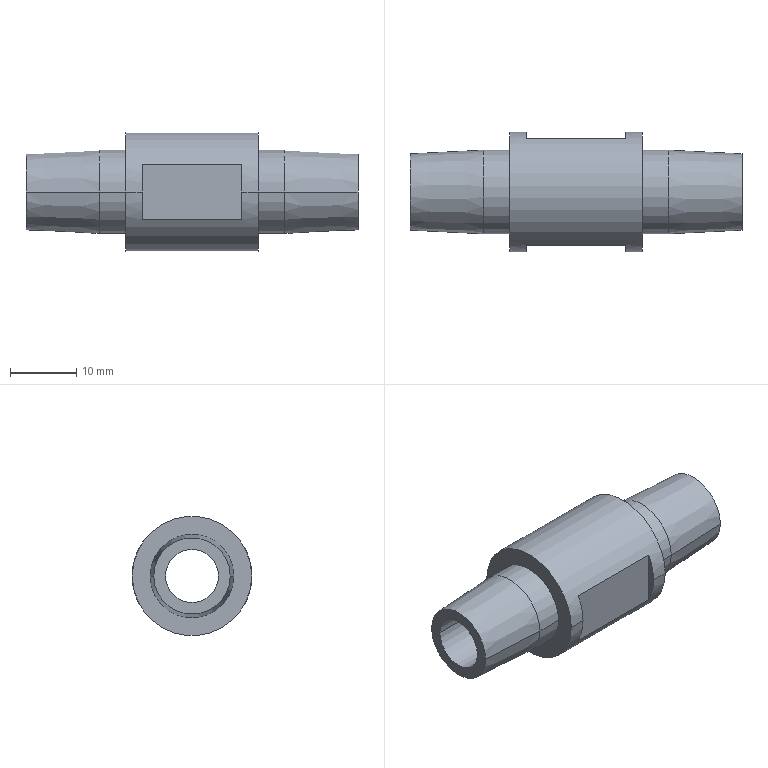Part | SolidWorks | features ICE 1, Revolution 1 | 1 solid | 22 faces | box 50 x 18 x 18 mm | volume 5917 mm3 | plane 10 | cylinder 8 | cone 4 | commonest cylinder face diameters 12.6 x4 8 x2 18 x2
STEP:
#1=CARTESIAN_POINT('',(15.,-6.3,0.));
#2=VERTEX_POINT('',#1);
#3=CARTESIAN_POINT('',(15.,6.3,0.));
#4=VERTEX_POINT('',#3);
#5=CARTESIAN_POINT('',(15.,0.,0.));
#6=DIRECTION('',(-1.,0.,0.));
#7=DIRECTION('',(0.,-1.,0.));
#8=AXIS2_PLACEMENT_3D('',#5,#6,#7);
#9=CIRCLE('',#8,6.3);
#10=EDGE_CURVE('',#2,#4,#9,.T.);
#11=ORIENTED_EDGE('',*,*,#10,.T.);
#12=CARTESIAN_POINT('',(11.,6.3,0.));
#13=VERTEX_POINT('',#12);
#14=CARTESIAN_POINT('',(0.,6.3,0.));
#15=DIRECTION('',(-1.,0.,0.));
#16=VECTOR('',#15,1000.);
#17=LINE('',#14,#16);
#18=EDGE_CURVE('',#4,#13,#17,.T.);
#19=ORIENTED_EDGE('',*,*,#18,.T.);
#20=CARTESIAN_POINT('',(11.,-6.3,0.));
#21=VERTEX_POINT('',#20);
#22=CARTESIAN_POINT('',(11.,0.,0.));
#23=DIRECTION('',(-1.,0.,0.));
#24=DIRECTION('',(0.,-1.,0.));
#25=AXIS2_PLACEMENT_3D('',#22,#23,#24);
#26=CIRCLE('',#25,6.3);
#27=EDGE_CURVE('',#21,#13,#26,.T.);
#28=ORIENTED_EDGE('',*,*,#27,.F.);
#29=CARTESIAN_POINT('',(0.,-6.3,0.));
#30=DIRECTION('',(-1.,0.,0.));
#31=VECTOR('',#30,1000.);
#32=LINE('',#29,#31);
#33=EDGE_CURVE('',#2,#21,#32,.T.);
#34=ORIENTED_EDGE('',*,*,#33,.F.);
#35=EDGE_LOOP('',(#11,#19,#28,#34));
#36=FACE_OUTER_BOUND('',#35,.T.);
#37=CARTESIAN_POINT('',(0.,0.,0.));
#38=DIRECTION('',(-1.,0.,0.));
#39=DIRECTION('',(0.,-1.,0.));
#40=AXIS2_PLACEMENT_3D('',#37,#38,#39);
#41=CYLINDRICAL_SURFACE('',#40,6.3);
#42=ADVANCED_FACE('',(#36),#41,.T.);
#43=CARTESIAN_POINT('',(0.,-5.75,0.));
#44=VERTEX_POINT('',#43);
#45=CARTESIAN_POINT('',(0.,5.75,0.));
#46=VERTEX_POINT('',#45);
#47=CARTESIAN_POINT('',(0.,0.,0.));
#48=DIRECTION('',(-1.,0.,0.));
#49=DIRECTION('',(0.,-1.,0.));
#50=AXIS2_PLACEMENT_3D('',#47,#48,#49);
#51=CIRCLE('',#50,5.75);
#52=EDGE_CURVE('',#44,#46,#51,.T.);
#53=ORIENTED_EDGE('',*,*,#52,.F.);
#54=CARTESIAN_POINT('',(11.,-6.3,0.));
#55=DIRECTION('',(0.9988,-0.04994,0.));
#56=VECTOR('',#55,1000.);
#57=LINE('',#54,#56);
#58=EDGE_CURVE('',#44,#21,#57,.T.);
#59=ORIENTED_EDGE('',*,*,#58,.T.);
#60=ORIENTED_EDGE('',*,*,#27,.T.);
#61=CARTESIAN_POINT('',(11.,6.3,0.));
#62=DIRECTION('',(0.9988,0.04994,0.));
#63=VECTOR('',#62,1000.);
#64=LINE('',#61,#63);
#65=EDGE_CURVE('',#46,#13,#64,.T.);
#66=ORIENTED_EDGE('',*,*,#65,.F.);
#67=EDGE_LOOP('',(#53,#59,#60,#66));
#68=FACE_OUTER_BOUND('',#67,.T.);
#69=CARTESIAN_POINT('',(11.,0.,0.));
#70=DIRECTION('',(1.,0.,0.));
#71=DIRECTION('',(0.,1.,0.));
#72=AXIS2_PLACEMENT_3D('',#69,#70,#71);
#73=CONICAL_SURFACE('',#72,6.3,0.04996);
#74=ADVANCED_FACE('',(#68),#73,.T.);
#75=CARTESIAN_POINT('',(50.,4.,0.));
#76=VERTEX_POINT('',#75);
#77=CARTESIAN_POINT('',(50.,-4.,0.));
#78=VERTEX_POINT('',#77);
#79=CARTESIAN_POINT('',(50.,0.,0.));
#80=DIRECTION('',(-1.,0.,0.));
#81=DIRECTION('',(0.,-1.,0.));
#82=AXIS2_PLACEMENT_3D('',#79,#80,#81);
#83=CIRCLE('',#82,4.);
#84=EDGE_CURVE('',#76,#78,#83,.T.);
#85=ORIENTED_EDGE('',*,*,#84,.F.);
#86=CARTESIAN_POINT('',(0.,4.,0.));
#87=VERTEX_POINT('',#86);
#88=CARTESIAN_POINT('',(0.,4.,0.));
#89=DIRECTION('',(-1.,0.,0.));
#90=VECTOR('',#89,1000.);
#91=LINE('',#88,#90);
#92=EDGE_CURVE('',#76,#87,#91,.T.);
#93=ORIENTED_EDGE('',*,*,#92,.T.);
#94=CARTESIAN_POINT('',(0.,-4.,0.));
#95=VERTEX_POINT('',#94);
#96=CARTESIAN_POINT('',(0.,0.,0.));
#97=DIRECTION('',(-1.,0.,0.));
#98=DIRECTION('',(0.,-1.,0.));
#99=AXIS2_PLACEMENT_3D('',#96,#97,#98);
#100=CIRCLE('',#99,4.);
#101=EDGE_CURVE('',#87,#95,#100,.T.);
#102=ORIENTED_EDGE('',*,*,#101,.T.);
#103=CARTESIAN_POINT('',(0.,-4.,0.));
#104=DIRECTION('',(-1.,0.,0.));
#105=VECTOR('',#104,1000.);
#106=LINE('',#103,#105);
#107=EDGE_CURVE('',#78,#95,#106,.T.);
#108=ORIENTED_EDGE('',*,*,#107,.F.);
#109=EDGE_LOOP('',(#85,#93,#102,#108));
#110=FACE_OUTER_BOUND('',#109,.T.);
#111=CARTESIAN_POINT('',(0.,0.,0.));
#112=DIRECTION('',(-1.,0.,0.));
#113=DIRECTION('',(0.,-1.,0.));
#114=AXIS2_PLACEMENT_3D('',#111,#112,#113);
#115=CYLINDRICAL_SURFACE('',#114,4.);
#116=ADVANCED_FACE('',(#110),#115,.F.);
#117=CARTESIAN_POINT('',(50.,-5.75,0.));
#118=VERTEX_POINT('',#117);
#119=CARTESIAN_POINT('',(50.,5.75,0.));
#120=VERTEX_POINT('',#119);
#121=CARTESIAN_POINT('',(50.,0.,0.));
#122=DIRECTION('',(-1.,0.,0.));
#123=DIRECTION('',(0.,-1.,0.));
#124=AXIS2_PLACEMENT_3D('',#121,#122,#123);
#125=CIRCLE('',#124,5.75);
#126=EDGE_CURVE('',#118,#120,#125,.T.);
#127=ORIENTED_EDGE('',*,*,#126,.T.);
#128=CARTESIAN_POINT('',(39.,6.3,0.));
#129=VERTEX_POINT('',#128);
#130=CARTESIAN_POINT('',(50.,5.75,0.));
#131=DIRECTION('',(-0.9988,0.04994,0.));
#132=VECTOR('',#131,1000.);
#133=LINE('',#130,#132);
#134=EDGE_CURVE('',#120,#129,#133,.T.);
#135=ORIENTED_EDGE('',*,*,#134,.T.);
#136=CARTESIAN_POINT('',(39.,-6.3,0.));
#137=VERTEX_POINT('',#136);
#138=CARTESIAN_POINT('',(39.,0.,0.));
#139=DIRECTION('',(-1.,0.,0.));
#140=DIRECTION('',(0.,-1.,0.));
#141=AXIS2_PLACEMENT_3D('',#138,#139,#140);
#142=CIRCLE('',#141,6.3);
#143=EDGE_CURVE('',#137,#129,#142,.T.);
#144=ORIENTED_EDGE('',*,*,#143,.F.);
#145=CARTESIAN_POINT('',(50.,-5.75,0.));
#146=DIRECTION('',(-0.9988,-0.04994,0.));
#147=VECTOR('',#146,1000.);
#148=LINE('',#145,#147);
#149=EDGE_CURVE('',#118,#137,#148,.T.);
#150=ORIENTED_EDGE('',*,*,#149,.F.);
#151=EDGE_LOOP('',(#127,#135,#144,#150));
#152=FACE_OUTER_BOUND('',#151,.T.);
#153=CARTESIAN_POINT('',(50.,0.,0.));
#154=DIRECTION('',(-1.,0.,0.));
#155=DIRECTION('',(0.,-1.,0.));
#156=AXIS2_PLACEMENT_3D('',#153,#154,#155);
#157=CONICAL_SURFACE('',#156,5.75,0.04996);
#158=ADVANCED_FACE('',(#152),#157,.T.);
#159=ORIENTED_EDGE('',*,*,#143,.T.);
#160=CARTESIAN_POINT('',(35.,6.3,0.));
#161=VERTEX_POINT('',#160);
#162=CARTESIAN_POINT('',(0.,6.3,0.));
#163=DIRECTION('',(-1.,0.,0.));
#164=VECTOR('',#163,1000.);
#165=LINE('',#162,#164);
#166=EDGE_CURVE('',#129,#161,#165,.T.);
#167=ORIENTED_EDGE('',*,*,#166,.T.);
#168=CARTESIAN_POINT('',(35.,-6.3,0.));
#169=VERTEX_POINT('',#168);
#170=CARTESIAN_POINT('',(35.,0.,0.));
#171=DIRECTION('',(-1.,0.,0.));
#172=DIRECTION('',(0.,-1.,0.));
#173=AXIS2_PLACEMENT_3D('',#170,#171,#172);
#174=CIRCLE('',#173,6.3);
#175=EDGE_CURVE('',#169,#161,#174,.T.);
#176=ORIENTED_EDGE('',*,*,#175,.F.);
#177=CARTESIAN_POINT('',(0.,-6.3,0.));
#178=DIRECTION('',(-1.,0.,0.));
#179=VECTOR('',#178,1000.);
#180=LINE('',#177,#179);
#181=EDGE_CURVE('',#137,#169,#180,.T.);
#182=ORIENTED_EDGE('',*,*,#181,.F.);
#183=EDGE_LOOP('',(#159,#167,#176,#182));
#184=FACE_OUTER_BOUND('',#183,.T.);
#185=CARTESIAN_POINT('',(0.,0.,0.));
#186=DIRECTION('',(-1.,0.,0.));
#187=DIRECTION('',(0.,-1.,0.));
#188=AXIS2_PLACEMENT_3D('',#185,#186,#187);
#189=CYLINDRICAL_SURFACE('',#188,6.3);
#190=ADVANCED_FACE('',(#184),#189,.T.);
#191=CARTESIAN_POINT('',(35.,-9.,0.));
#192=VERTEX_POINT('',#191);
#193=CARTESIAN_POINT('',(35.,9.,0.));
#194=VERTEX_POINT('',#193);
#195=CARTESIAN_POINT('',(35.,0.,0.));
#196=DIRECTION('',(-1.,0.,0.));
#197=DIRECTION('',(0.,-1.,0.));
#198=AXIS2_PLACEMENT_3D('',#195,#196,#197);
#199=CIRCLE('',#198,9.);
#200=EDGE_CURVE('',#192,#194,#199,.T.);
#201=ORIENTED_EDGE('',*,*,#200,.T.);
#202=CARTESIAN_POINT('',(32.5,9.,0.));
#203=VERTEX_POINT('',#202);
#204=CARTESIAN_POINT('',(0.,9.,0.));
#205=DIRECTION('',(-1.,0.,0.));
#206=VECTOR('',#205,1000.);
#207=LINE('',#204,#206);
#208=EDGE_CURVE('',#194,#203,#207,.T.);
#209=ORIENTED_EDGE('',*,*,#208,.T.);
#210=CARTESIAN_POINT('',(32.5,8.,4.123));
#211=VERTEX_POINT('',#210);
#212=CARTESIAN_POINT('',(32.5,0.,0.));
#213=DIRECTION('',(-1.,0.,0.));
#214=DIRECTION('',(0.,-1.,0.));
#215=AXIS2_PLACEMENT_3D('',#212,#213,#214);
#216=CIRCLE('',#215,9.);
#217=EDGE_CURVE('',#211,#203,#216,.T.);
#218=ORIENTED_EDGE('',*,*,#217,.F.);
#219=CARTESIAN_POINT('',(17.5,8.,4.123));
#220=VERTEX_POINT('',#219);
#221=CARTESIAN_POINT('',(0.,8.,4.123));
#222=DIRECTION('',(1.,0.,0.));
#223=VECTOR('',#222,1000.);
#224=LINE('',#221,#223);
#225=EDGE_CURVE('',#220,#211,#224,.T.);
#226=ORIENTED_EDGE('',*,*,#225,.F.);
#227=CARTESIAN_POINT('',(17.5,9.,0.));
#228=VERTEX_POINT('',#227);
#229=CARTESIAN_POINT('',(17.5,0.,0.));
#230=DIRECTION('',(-1.,0.,0.));
#231=DIRECTION('',(0.,-1.,0.));
#232=AXIS2_PLACEMENT_3D('',#229,#230,#231);
#233=CIRCLE('',#232,9.);
#234=EDGE_CURVE('',#220,#228,#233,.T.);
#235=ORIENTED_EDGE('',*,*,#234,.T.);
#236=CARTESIAN_POINT('',(15.,9.,0.));
#237=VERTEX_POINT('',#236);
#238=CARTESIAN_POINT('',(0.,9.,0.));
#239=DIRECTION('',(-1.,0.,0.));
#240=VECTOR('',#239,1000.);
#241=LINE('',#238,#240);
#242=EDGE_CURVE('',#228,#237,#241,.T.);
#243=ORIENTED_EDGE('',*,*,#242,.T.);
#244=CARTESIAN_POINT('',(15.,-9.,0.));
#245=VERTEX_POINT('',#244);
#246=CARTESIAN_POINT('',(15.,0.,0.));
#247=DIRECTION('',(-1.,0.,0.));
#248=DIRECTION('',(0.,-1.,0.));
#249=AXIS2_PLACEMENT_3D('',#246,#247,#248);
#250=CIRCLE('',#249,9.);
#251=EDGE_CURVE('',#245,#237,#250,.T.);
#252=ORIENTED_EDGE('',*,*,#251,.F.);
#253=CARTESIAN_POINT('',(17.5,-9.,0.));
#254=VERTEX_POINT('',#253);
#255=CARTESIAN_POINT('',(0.,-9.,0.));
#256=DIRECTION('',(-1.,0.,0.));
#257=VECTOR('',#256,1000.);
#258=LINE('',#255,#257);
#259=EDGE_CURVE('',#254,#245,#258,.T.);
#260=ORIENTED_EDGE('',*,*,#259,.F.);
#261=CARTESIAN_POINT('',(17.5,-8.,4.123));
#262=VERTEX_POINT('',#261);
#263=CARTESIAN_POINT('',(17.5,0.,0.));
#264=DIRECTION('',(-1.,0.,0.));
#265=DIRECTION('',(0.,-1.,0.));
#266=AXIS2_PLACEMENT_3D('',#263,#264,#265);
#267=CIRCLE('',#266,9.);
#268=EDGE_CURVE('',#254,#262,#267,.T.);
#269=ORIENTED_EDGE('',*,*,#268,.T.);
#270=CARTESIAN_POINT('',(32.5,-8.,4.123));
#271=VERTEX_POINT('',#270);
#272=CARTESIAN_POINT('',(0.,-8.,4.123));
#273=DIRECTION('',(-1.,0.,0.));
#274=VECTOR('',#273,1000.);
#275=LINE('',#272,#274);
#276=EDGE_CURVE('',#271,#262,#275,.T.);
#277=ORIENTED_EDGE('',*,*,#276,.F.);
#278=CARTESIAN_POINT('',(32.5,-9.,0.));
#279=VERTEX_POINT('',#278);
#280=CARTESIAN_POINT('',(32.5,0.,0.));
#281=DIRECTION('',(-1.,0.,0.));
#282=DIRECTION('',(0.,-1.,0.));
#283=AXIS2_PLACEMENT_3D('',#280,#281,#282);
#284=CIRCLE('',#283,9.);
#285=EDGE_CURVE('',#279,#271,#284,.T.);
#286=ORIENTED_EDGE('',*,*,#285,.F.);
#287=CARTESIAN_POINT('',(0.,-9.,0.));
#288=DIRECTION('',(-1.,0.,0.));
#289=VECTOR('',#288,1000.);
#290=LINE('',#287,#289);
#291=EDGE_CURVE('',#192,#279,#290,.T.);
#292=ORIENTED_EDGE('',*,*,#291,.F.);
#293=EDGE_LOOP('',(#201,#209,#218,#226,#235,#243,#252,#260,#269,#277,#286,#292));
#294=FACE_OUTER_BOUND('',#293,.T.);
#295=CARTESIAN_POINT('',(0.,0.,0.));
#296=DIRECTION('',(-1.,0.,0.));
#297=DIRECTION('',(0.,-1.,0.));
#298=AXIS2_PLACEMENT_3D('',#295,#296,#297);
#299=CYLINDRICAL_SURFACE('',#298,9.);
#300=ADVANCED_FACE('',(#294),#299,.T.);
#301=ORIENTED_EDGE('',*,*,#208,.F.);
#302=CARTESIAN_POINT('',(35.,0.,0.));
#303=DIRECTION('',(-1.,0.,0.));
#304=DIRECTION('',(0.,-1.,0.));
#305=AXIS2_PLACEMENT_3D('',#302,#303,#304);
#306=CIRCLE('',#305,9.);
#307=EDGE_CURVE('',#194,#192,#306,.T.);
#308=ORIENTED_EDGE('',*,*,#307,.T.);
#309=ORIENTED_EDGE('',*,*,#291,.T.);
#310=CARTESIAN_POINT('',(32.5,-8.,-4.123));
#311=VERTEX_POINT('',#310);
#312=CARTESIAN_POINT('',(32.5,0.,0.));
#313=DIRECTION('',(-1.,0.,0.));
#314=DIRECTION('',(0.,-1.,0.));
#315=AXIS2_PLACEMENT_3D('',#312,#313,#314);
#316=CIRCLE('',#315,9.);
#317=EDGE_CURVE('',#311,#279,#316,.T.);
#318=ORIENTED_EDGE('',*,*,#317,.F.);
#319=CARTESIAN_POINT('',(17.5,-8.,-4.123));
#320=VERTEX_POINT('',#319);
#321=CARTESIAN_POINT('',(0.,-8.,-4.123));
#322=DIRECTION('',(1.,0.,0.));
#323=VECTOR('',#322,1000.);
#324=LINE('',#321,#323);
#325=EDGE_CURVE('',#320,#311,#324,.T.);
#326=ORIENTED_EDGE('',*,*,#325,.F.);
#327=CARTESIAN_POINT('',(17.5,0.,0.));
#328=DIRECTION('',(-1.,0.,0.));
#329=DIRECTION('',(0.,-1.,0.));
#330=AXIS2_PLACEMENT_3D('',#327,#328,#329);
#331=CIRCLE('',#330,9.);
#332=EDGE_CURVE('',#320,#254,#331,.T.);
#333=ORIENTED_EDGE('',*,*,#332,.T.);
#334=ORIENTED_EDGE('',*,*,#259,.T.);
#335=CARTESIAN_POINT('',(15.,0.,0.));
#336=DIRECTION('',(-1.,0.,0.));
#337=DIRECTION('',(0.,-1.,0.));
#338=AXIS2_PLACEMENT_3D('',#335,#336,#337);
#339=CIRCLE('',#338,9.);
#340=EDGE_CURVE('',#237,#245,#339,.T.);
#341=ORIENTED_EDGE('',*,*,#340,.F.);
#342=ORIENTED_EDGE('',*,*,#242,.F.);
#343=CARTESIAN_POINT('',(17.5,8.,-4.123));
#344=VERTEX_POINT('',#343);
#345=CARTESIAN_POINT('',(17.5,0.,0.));
#346=DIRECTION('',(-1.,0.,0.));
#347=DIRECTION('',(0.,-1.,0.));
#348=AXIS2_PLACEMENT_3D('',#345,#346,#347);
#349=CIRCLE('',#348,9.);
#350=EDGE_CURVE('',#228,#344,#349,.T.);
#351=ORIENTED_EDGE('',*,*,#350,.T.);
#352=CARTESIAN_POINT('',(32.5,8.,-4.123));
#353=VERTEX_POINT('',#352);
#354=CARTESIAN_POINT('',(0.,8.,-4.123));
#355=DIRECTION('',(-1.,0.,0.));
#356=VECTOR('',#355,1000.);
#357=LINE('',#354,#356);
#358=EDGE_CURVE('',#353,#344,#357,.T.);
#359=ORIENTED_EDGE('',*,*,#358,.F.);
#360=CARTESIAN_POINT('',(32.5,0.,0.));
#361=DIRECTION('',(-1.,0.,0.));
#362=DIRECTION('',(0.,-1.,0.));
#363=AXIS2_PLACEMENT_3D('',#360,#361,#362);
#364=CIRCLE('',#363,9.);
#365=EDGE_CURVE('',#203,#353,#364,.T.);
#366=ORIENTED_EDGE('',*,*,#365,.F.);
#367=EDGE_LOOP('',(#301,#308,#309,#318,#326,#333,#334,#341,#342,#351,#359,#366));
#368=FACE_OUTER_BOUND('',#367,.T.);
#369=CARTESIAN_POINT('',(0.,0.,0.));
#370=DIRECTION('',(-1.,0.,0.));
#371=DIRECTION('',(0.,-1.,0.));
#372=AXIS2_PLACEMENT_3D('',#369,#370,#371);
#373=CYLINDRICAL_SURFACE('',#372,9.);
#374=ADVANCED_FACE('',(#368),#373,.T.);
#375=ORIENTED_EDGE('',*,*,#166,.F.);
#376=CARTESIAN_POINT('',(39.,0.,0.));
#377=DIRECTION('',(-1.,0.,0.));
#378=DIRECTION('',(0.,-1.,0.));
#379=AXIS2_PLACEMENT_3D('',#376,#377,#378);
#380=CIRCLE('',#379,6.3);
#381=EDGE_CURVE('',#129,#137,#380,.T.);
#382=ORIENTED_EDGE('',*,*,#381,.T.);
#383=ORIENTED_EDGE('',*,*,#181,.T.);
#384=CARTESIAN_POINT('',(35.,0.,0.));
#385=DIRECTION('',(-1.,0.,0.));
#386=DIRECTION('',(0.,-1.,0.));
#387=AXIS2_PLACEMENT_3D('',#384,#385,#386);
#388=CIRCLE('',#387,6.3);
#389=EDGE_CURVE('',#161,#169,#388,.T.);
#390=ORIENTED_EDGE('',*,*,#389,.F.);
#391=EDGE_LOOP('',(#375,#382,#383,#390));
#392=FACE_OUTER_BOUND('',#391,.T.);
#393=CARTESIAN_POINT('',(0.,0.,0.));
#394=DIRECTION('',(-1.,0.,0.));
#395=DIRECTION('',(0.,-1.,0.));
#396=AXIS2_PLACEMENT_3D('',#393,#394,#395);
#397=CYLINDRICAL_SURFACE('',#396,6.3);
#398=ADVANCED_FACE('',(#392),#397,.T.);
#399=ORIENTED_EDGE('',*,*,#134,.F.);
#400=CARTESIAN_POINT('',(50.,0.,0.));
#401=DIRECTION('',(-1.,0.,0.));
#402=DIRECTION('',(0.,-1.,0.));
#403=AXIS2_PLACEMENT_3D('',#400,#401,#402);
#404=CIRCLE('',#403,5.75);
#405=EDGE_CURVE('',#120,#118,#404,.T.);
#406=ORIENTED_EDGE('',*,*,#405,.T.);
#407=ORIENTED_EDGE('',*,*,#149,.T.);
#408=ORIENTED_EDGE('',*,*,#381,.F.);
#409=EDGE_LOOP('',(#399,#406,#407,#408));
#410=FACE_OUTER_BOUND('',#409,.T.);
#411=CARTESIAN_POINT('',(50.,0.,0.));
#412=DIRECTION('',(-1.,0.,0.));
#413=DIRECTION('',(0.,-1.,0.));
#414=AXIS2_PLACEMENT_3D('',#411,#412,#413);
#415=CONICAL_SURFACE('',#414,5.75,0.04996);
#416=ADVANCED_FACE('',(#410),#415,.T.);
#417=ORIENTED_EDGE('',*,*,#126,.F.);
#418=ORIENTED_EDGE('',*,*,#405,.F.);
#419=EDGE_LOOP('',(#417,#418));
#420=FACE_OUTER_BOUND('',#419,.T.);
#421=CARTESIAN_POINT('',(50.,0.,0.));
#422=DIRECTION('',(-1.,0.,0.));
#423=DIRECTION('',(0.,-1.,0.));
#424=AXIS2_PLACEMENT_3D('',#421,#422,#423);
#425=CIRCLE('',#424,4.);
#426=EDGE_CURVE('',#78,#76,#425,.T.);
#427=ORIENTED_EDGE('',*,*,#426,.T.);
#428=ORIENTED_EDGE('',*,*,#84,.T.);
#429=EDGE_LOOP('',(#427,#428));
#430=FACE_BOUND('',#429,.T.);
#431=CARTESIAN_POINT('',(50.,4.,0.));
#432=DIRECTION('',(-1.,0.,0.));
#433=DIRECTION('',(0.,-1.,0.));
#434=AXIS2_PLACEMENT_3D('',#431,#432,#433);
#435=PLANE('',#434);
#436=ADVANCED_FACE('',(#420,#430),#435,.F.);
#437=ORIENTED_EDGE('',*,*,#92,.F.);
#438=ORIENTED_EDGE('',*,*,#426,.F.);
#439=ORIENTED_EDGE('',*,*,#107,.T.);
#440=CARTESIAN_POINT('',(0.,0.,0.));
#441=DIRECTION('',(-1.,0.,0.));
#442=DIRECTION('',(0.,-1.,0.));
#443=AXIS2_PLACEMENT_3D('',#440,#441,#442);
#444=CIRCLE('',#443,4.);
#445=EDGE_CURVE('',#95,#87,#444,.T.);
#446=ORIENTED_EDGE('',*,*,#445,.T.);
#447=EDGE_LOOP('',(#437,#438,#439,#446));
#448=FACE_OUTER_BOUND('',#447,.T.);
#449=CARTESIAN_POINT('',(0.,0.,0.));
#450=DIRECTION('',(-1.,0.,0.));
#451=DIRECTION('',(0.,-1.,0.));
#452=AXIS2_PLACEMENT_3D('',#449,#450,#451);
#453=CYLINDRICAL_SURFACE('',#452,4.);
#454=ADVANCED_FACE('',(#448),#453,.F.);
#455=ORIENTED_EDGE('',*,*,#445,.F.);
#456=ORIENTED_EDGE('',*,*,#101,.F.);
#457=EDGE_LOOP('',(#455,#456));
#458=FACE_BOUND('',#457,.T.);
#459=CARTESIAN_POINT('',(0.,0.,0.));
#460=DIRECTION('',(-1.,0.,0.));
#461=DIRECTION('',(0.,-1.,0.));
#462=AXIS2_PLACEMENT_3D('',#459,#460,#461);
#463=CIRCLE('',#462,5.75);
#464=EDGE_CURVE('',#46,#44,#463,.T.);
#465=ORIENTED_EDGE('',*,*,#464,.T.);
#466=ORIENTED_EDGE('',*,*,#52,.T.);
#467=EDGE_LOOP('',(#465,#466));
#468=FACE_OUTER_BOUND('',#467,.T.);
#469=CARTESIAN_POINT('',(0.,4.,0.));
#470=DIRECTION('',(1.,0.,0.));
#471=DIRECTION('',(0.,1.,0.));
#472=AXIS2_PLACEMENT_3D('',#469,#470,#471);
#473=PLANE('',#472);
#474=ADVANCED_FACE('',(#458,#468),#473,.F.);
#475=ORIENTED_EDGE('',*,*,#58,.F.);
#476=ORIENTED_EDGE('',*,*,#464,.F.);
#477=ORIENTED_EDGE('',*,*,#65,.T.);
#478=CARTESIAN_POINT('',(11.,0.,0.));
#479=DIRECTION('',(-1.,0.,0.));
#480=DIRECTION('',(0.,-1.,0.));
#481=AXIS2_PLACEMENT_3D('',#478,#479,#480);
#482=CIRCLE('',#481,6.3);
#483=EDGE_CURVE('',#13,#21,#482,.T.);
#484=ORIENTED_EDGE('',*,*,#483,.T.);
#485=EDGE_LOOP('',(#475,#476,#477,#484));
#486=FACE_OUTER_BOUND('',#485,.T.);
#487=CARTESIAN_POINT('',(11.,0.,0.));
#488=DIRECTION('',(1.,0.,0.));
#489=DIRECTION('',(0.,1.,0.));
#490=AXIS2_PLACEMENT_3D('',#487,#488,#489);
#491=CONICAL_SURFACE('',#490,6.3,0.04996);
#492=ADVANCED_FACE('',(#486),#491,.T.);
#493=ORIENTED_EDGE('',*,*,#18,.F.);
#494=CARTESIAN_POINT('',(15.,0.,0.));
#495=DIRECTION('',(-1.,0.,0.));
#496=DIRECTION('',(0.,-1.,0.));
#497=AXIS2_PLACEMENT_3D('',#494,#495,#496);
#498=CIRCLE('',#497,6.3);
#499=EDGE_CURVE('',#4,#2,#498,.T.);
#500=ORIENTED_EDGE('',*,*,#499,.T.);
#501=ORIENTED_EDGE('',*,*,#33,.T.);
#502=ORIENTED_EDGE('',*,*,#483,.F.);
#503=EDGE_LOOP('',(#493,#500,#501,#502));
#504=FACE_OUTER_BOUND('',#503,.T.);
#505=CARTESIAN_POINT('',(0.,0.,0.));
#506=DIRECTION('',(-1.,0.,0.));
#507=DIRECTION('',(0.,-1.,0.));
#508=AXIS2_PLACEMENT_3D('',#505,#506,#507);
#509=CYLINDRICAL_SURFACE('',#508,6.3);
#510=ADVANCED_FACE('',(#504),#509,.T.);
#511=ORIENTED_EDGE('',*,*,#10,.F.);
#512=ORIENTED_EDGE('',*,*,#499,.F.);
#513=EDGE_LOOP('',(#511,#512));
#514=FACE_BOUND('',#513,.T.);
#515=ORIENTED_EDGE('',*,*,#251,.T.);
#516=ORIENTED_EDGE('',*,*,#340,.T.);
#517=EDGE_LOOP('',(#515,#516));
#518=FACE_OUTER_BOUND('',#517,.T.);
#519=CARTESIAN_POINT('',(15.,6.3,0.));
#520=DIRECTION('',(1.,0.,0.));
#521=DIRECTION('',(0.,1.,0.));
#522=AXIS2_PLACEMENT_3D('',#519,#520,#521);
#523=PLANE('',#522);
#524=ADVANCED_FACE('',(#514,#518),#523,.F.);
#525=ORIENTED_EDGE('',*,*,#200,.F.);
#526=ORIENTED_EDGE('',*,*,#307,.F.);
#527=EDGE_LOOP('',(#525,#526));
#528=FACE_OUTER_BOUND('',#527,.T.);
#529=ORIENTED_EDGE('',*,*,#175,.T.);
#530=ORIENTED_EDGE('',*,*,#389,.T.);
#531=EDGE_LOOP('',(#529,#530));
#532=FACE_BOUND('',#531,.T.);
#533=CARTESIAN_POINT('',(35.,6.3,0.));
#534=DIRECTION('',(-1.,0.,0.));
#535=DIRECTION('',(0.,-1.,0.));
#536=AXIS2_PLACEMENT_3D('',#533,#534,#535);
#537=PLANE('',#536);
#538=ADVANCED_FACE('',(#528,#532),#537,.F.);
#539=ORIENTED_EDGE('',*,*,#358,.T.);
#540=CARTESIAN_POINT('',(17.5,8.,-10.453));
#541=DIRECTION('',(0.,0.,-1.));
#542=VECTOR('',#541,1000.);
#543=LINE('',#540,#542);
#544=EDGE_CURVE('',#220,#344,#543,.T.);
#545=ORIENTED_EDGE('',*,*,#544,.F.);
#546=ORIENTED_EDGE('',*,*,#225,.T.);
#547=CARTESIAN_POINT('',(32.5,8.,-10.453));
#548=DIRECTION('',(0.,0.,-1.));
#549=VECTOR('',#548,1000.);
#550=LINE('',#547,#549);
#551=EDGE_CURVE('',#211,#353,#550,.T.);
#552=ORIENTED_EDGE('',*,*,#551,.T.);
#553=EDGE_LOOP('',(#539,#545,#546,#552));
#554=FACE_OUTER_BOUND('',#553,.T.);
#555=CARTESIAN_POINT('',(32.5,8.,-10.453));
#556=DIRECTION('',(0.,1.,0.));
#557=DIRECTION('',(0.,0.,1.));
#558=AXIS2_PLACEMENT_3D('',#555,#556,#557);
#559=PLANE('',#558);
#560=ADVANCED_FACE('',(#554),#559,.T.);
#561=ORIENTED_EDGE('',*,*,#544,.T.);
#562=ORIENTED_EDGE('',*,*,#350,.F.);
#563=ORIENTED_EDGE('',*,*,#234,.F.);
#564=EDGE_LOOP('',(#561,#562,#563));
#565=FACE_OUTER_BOUND('',#564,.T.);
#566=CARTESIAN_POINT('',(17.5,0.,0.));
#567=DIRECTION('',(-1.,0.,0.));
#568=DIRECTION('',(0.,-1.,0.));
#569=AXIS2_PLACEMENT_3D('',#566,#567,#568);
#570=PLANE('',#569);
#571=ADVANCED_FACE('',(#565),#570,.F.);
#572=ORIENTED_EDGE('',*,*,#217,.T.);
#573=ORIENTED_EDGE('',*,*,#365,.T.);
#574=ORIENTED_EDGE('',*,*,#551,.F.);
#575=EDGE_LOOP('',(#572,#573,#574));
#576=FACE_OUTER_BOUND('',#575,.T.);
#577=CARTESIAN_POINT('',(32.5,0.,0.));
#578=DIRECTION('',(-1.,0.,0.));
#579=DIRECTION('',(0.,-1.,0.));
#580=AXIS2_PLACEMENT_3D('',#577,#578,#579);
#581=PLANE('',#580);
#582=ADVANCED_FACE('',(#576),#581,.T.);
#583=ORIENTED_EDGE('',*,*,#317,.T.);
#584=ORIENTED_EDGE('',*,*,#285,.T.);
#585=CARTESIAN_POINT('',(32.5,-8.,-10.453));
#586=DIRECTION('',(0.,0.,1.));
#587=VECTOR('',#586,1000.);
#588=LINE('',#585,#587);
#589=EDGE_CURVE('',#311,#271,#588,.T.);
#590=ORIENTED_EDGE('',*,*,#589,.F.);
#591=EDGE_LOOP('',(#583,#584,#590));
#592=FACE_OUTER_BOUND('',#591,.T.);
#593=CARTESIAN_POINT('',(32.5,0.,0.));
#594=DIRECTION('',(-1.,0.,0.));
#595=DIRECTION('',(0.,-1.,0.));
#596=AXIS2_PLACEMENT_3D('',#593,#594,#595);
#597=PLANE('',#596);
#598=ADVANCED_FACE('',(#592),#597,.T.);
#599=CARTESIAN_POINT('',(17.5,-8.,-10.453));
#600=DIRECTION('',(0.,0.,1.));
#601=VECTOR('',#600,1000.);
#602=LINE('',#599,#601);
#603=EDGE_CURVE('',#320,#262,#602,.T.);
#604=ORIENTED_EDGE('',*,*,#603,.T.);
#605=ORIENTED_EDGE('',*,*,#268,.F.);
#606=ORIENTED_EDGE('',*,*,#332,.F.);
#607=EDGE_LOOP('',(#604,#605,#606));
#608=FACE_OUTER_BOUND('',#607,.T.);
#609=CARTESIAN_POINT('',(17.5,0.,0.));
#610=DIRECTION('',(-1.,0.,0.));
#611=DIRECTION('',(0.,-1.,0.));
#612=AXIS2_PLACEMENT_3D('',#609,#610,#611);
#613=PLANE('',#612);
#614=ADVANCED_FACE('',(#608),#613,.F.);
#615=ORIENTED_EDGE('',*,*,#276,.T.);
#616=ORIENTED_EDGE('',*,*,#603,.F.);
#617=ORIENTED_EDGE('',*,*,#325,.T.);
#618=ORIENTED_EDGE('',*,*,#589,.T.);
#619=EDGE_LOOP('',(#615,#616,#617,#618));
#620=FACE_OUTER_BOUND('',#619,.T.);
#621=CARTESIAN_POINT('',(32.5,-8.,-10.453));
#622=DIRECTION('',(0.,-1.,0.));
#623=DIRECTION('',(0.,0.,-1.));
#624=AXIS2_PLACEMENT_3D('',#621,#622,#623);
#625=PLANE('',#624);
#626=ADVANCED_FACE('',(#620),#625,.T.);
#627=CLOSED_SHELL('',(#42,#74,#116,#158,#190,#300,#374,#398,#416,#436,#454,#474,#492,#510,#524,#538,#560,#571,#582,#598,#614,#626));
#628=MANIFOLD_SOLID_BREP('',#627);
#629=CARTESIAN_POINT('',(0.,0.,0.));
#630=DIRECTION('',(0.,0.,1.));
#631=DIRECTION('',(1.,0.,0.));
#632=AXIS2_PLACEMENT_3D('',#629,#630,#631);
#633=(LENGTH_UNIT()NAMED_UNIT(*)SI_UNIT(.MILLI.,.METRE.));
#634=UNCERTAINTY_MEASURE_WITH_UNIT(LENGTH_MEASURE(0.00001),#633,'','');
#635=(NAMED_UNIT(*)PLANE_ANGLE_UNIT()SI_UNIT($,.RADIAN.));
#636=(NAMED_UNIT(*)SI_UNIT($,.STERADIAN.)SOLID_ANGLE_UNIT());
#637=(GEOMETRIC_REPRESENTATION_CONTEXT(3)GLOBAL_UNCERTAINTY_ASSIGNED_CONTEXT((#634))GLOBAL_UNIT_ASSIGNED_CONTEXT((#633,#635,#636))REPRESENTATION_CONTEXT('',''));
#638=ADVANCED_BREP_SHAPE_REPRESENTATION('',(#628,#632),#637);